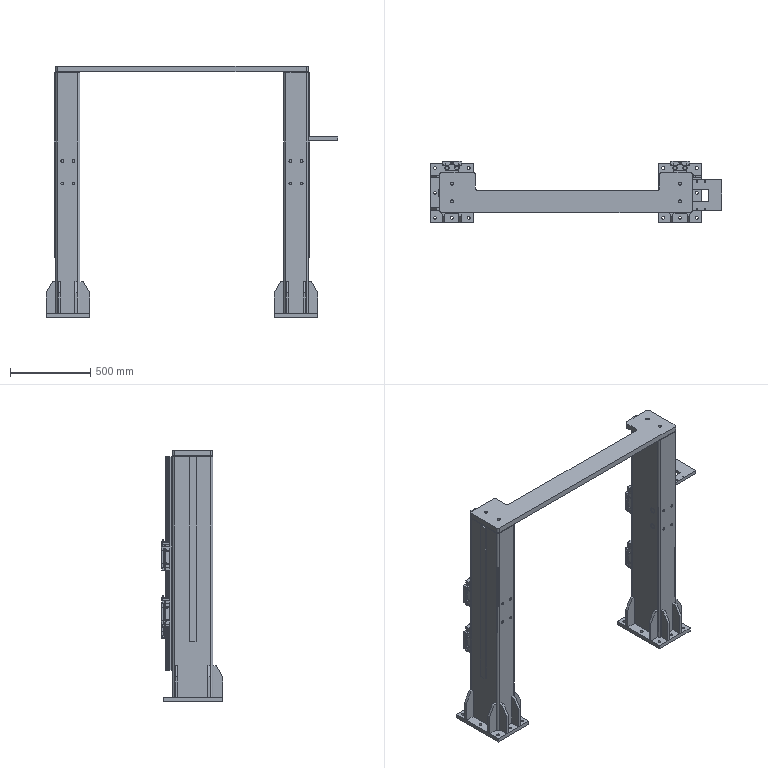Part | SolidWorks | 54 solids | 2498 faces | box 1815 x 380 x 1565 mm | volume 40801474 mm3 | plane 1556 | cylinder 710 | torus 100 | cone 92 | sphere 40 | commonest cylinder face diameters 3.924 x144 12 x104 20 x60 14 x52 6.06 x48 17.5 x48